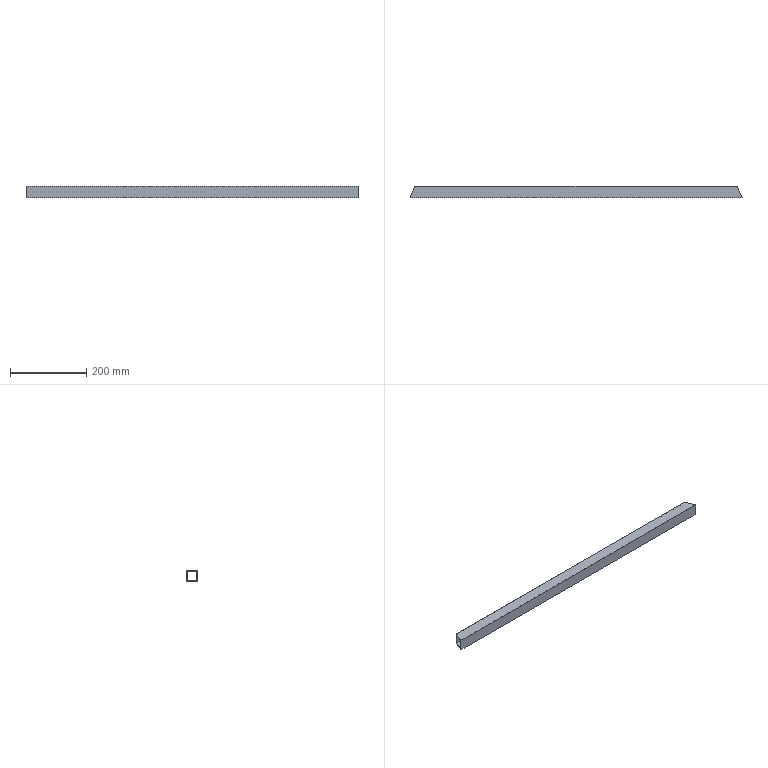Part | NX | features solid 2 | 1 solid | 10 faces | box 870 x 30 x 30 mm | volume 192096 mm3 | plane 10
STEP:
#1=CARTESIAN_POINT('',(422.574,270.,-110.));
#2=VERTEX_POINT('',#1);
#3=CARTESIAN_POINT('',(422.574,270.,-140.));
#4=VERTEX_POINT('',#3);
#5=CARTESIAN_POINT('',(422.574,270.,-110.));
#6=DIRECTION('',(0.,0.,-1.));
#7=VECTOR('',#6,1000.);
#8=LINE('',#5,#7);
#9=EDGE_CURVE('',#2,#4,#8,.T.);
#10=ORIENTED_EDGE('',*,*,#9,.T.);
#11=CARTESIAN_POINT('',(-422.574,270.,-140.));
#12=VERTEX_POINT('',#11);
#13=CARTESIAN_POINT('',(435.,270.,-140.));
#14=DIRECTION('',(-1.,0.,0.));
#15=VECTOR('',#14,1000.);
#16=LINE('',#13,#15);
#17=EDGE_CURVE('',#4,#12,#16,.T.);
#18=ORIENTED_EDGE('',*,*,#17,.T.);
#19=CARTESIAN_POINT('',(-422.574,270.,-110.));
#20=VERTEX_POINT('',#19);
#21=CARTESIAN_POINT('',(-422.574,270.,-110.));
#22=DIRECTION('',(0.,0.,-1.));
#23=VECTOR('',#22,1000.);
#24=LINE('',#21,#23);
#25=EDGE_CURVE('',#20,#12,#24,.T.);
#26=ORIENTED_EDGE('',*,*,#25,.F.);
#27=CARTESIAN_POINT('',(435.,270.,-110.));
#28=DIRECTION('',(-1.,0.,0.));
#29=VECTOR('',#28,1000.);
#30=LINE('',#27,#29);
#31=EDGE_CURVE('',#2,#20,#30,.T.);
#32=ORIENTED_EDGE('',*,*,#31,.F.);
#33=EDGE_LOOP('',(#10,#18,#26,#32));
#34=FACE_BOUND('',#33,.T.);
#35=CARTESIAN_POINT('',(435.,270.,-110.));
#36=DIRECTION('',(0.,1.,0.));
#37=DIRECTION('',(0.,0.,1.));
#38=AXIS2_PLACEMENT_3D('',#35,#36,#37);
#39=PLANE('',#38);
#40=ADVANCED_FACE('',(#34),#39,.T.);
#41=CARTESIAN_POINT('',(435.,240.,-140.));
#42=VERTEX_POINT('',#41);
#43=CARTESIAN_POINT('',(-435.,240.,-140.));
#44=VERTEX_POINT('',#43);
#45=CARTESIAN_POINT('',(435.,240.,-140.));
#46=DIRECTION('',(-1.,0.,0.));
#47=VECTOR('',#46,1000.);
#48=LINE('',#45,#47);
#49=EDGE_CURVE('',#42,#44,#48,.T.);
#50=ORIENTED_EDGE('',*,*,#49,.F.);
#51=CARTESIAN_POINT('',(435.,240.,-110.));
#52=VERTEX_POINT('',#51);
#53=CARTESIAN_POINT('',(435.,240.,-110.));
#54=DIRECTION('',(0.,0.,-1.));
#55=VECTOR('',#54,1000.);
#56=LINE('',#53,#55);
#57=EDGE_CURVE('',#52,#42,#56,.T.);
#58=ORIENTED_EDGE('',*,*,#57,.F.);
#59=CARTESIAN_POINT('',(-435.,240.,-110.));
#60=VERTEX_POINT('',#59);
#61=CARTESIAN_POINT('',(435.,240.,-110.));
#62=DIRECTION('',(-1.,0.,0.));
#63=VECTOR('',#62,1000.);
#64=LINE('',#61,#63);
#65=EDGE_CURVE('',#52,#60,#64,.T.);
#66=ORIENTED_EDGE('',*,*,#65,.T.);
#67=CARTESIAN_POINT('',(-435.,240.,-110.));
#68=DIRECTION('',(0.,0.,-1.));
#69=VECTOR('',#68,1000.);
#70=LINE('',#67,#69);
#71=EDGE_CURVE('',#60,#44,#70,.T.);
#72=ORIENTED_EDGE('',*,*,#71,.T.);
#73=EDGE_LOOP('',(#50,#58,#66,#72));
#74=FACE_BOUND('',#73,.T.);
#75=CARTESIAN_POINT('',(435.,240.,-110.));
#76=DIRECTION('',(0.,1.,0.));
#77=DIRECTION('',(0.,0.,1.));
#78=AXIS2_PLACEMENT_3D('',#75,#76,#77);
#79=PLANE('',#78);
#80=ADVANCED_FACE('',(#74),#79,.F.);
#81=ORIENTED_EDGE('',*,*,#31,.T.);
#82=CARTESIAN_POINT('',(-424.393,265.607,-110.));
#83=DIRECTION('',(-0.3827,-0.9239,0.));
#84=VECTOR('',#83,1000.);
#85=LINE('',#82,#84);
#86=EDGE_CURVE('',#20,#60,#85,.T.);
#87=ORIENTED_EDGE('',*,*,#86,.T.);
#88=ORIENTED_EDGE('',*,*,#65,.F.);
#89=CARTESIAN_POINT('',(424.393,265.607,-110.));
#90=DIRECTION('',(0.3827,-0.9239,0.));
#91=VECTOR('',#90,1000.);
#92=LINE('',#89,#91);
#93=EDGE_CURVE('',#2,#52,#92,.T.);
#94=ORIENTED_EDGE('',*,*,#93,.F.);
#95=EDGE_LOOP('',(#81,#87,#88,#94));
#96=FACE_BOUND('',#95,.T.);
#97=CARTESIAN_POINT('',(435.,270.,-110.));
#98=DIRECTION('',(0.,0.,-1.));
#99=DIRECTION('',(1.,0.,0.));
#100=AXIS2_PLACEMENT_3D('',#97,#98,#99);
#101=PLANE('',#100);
#102=ADVANCED_FACE('',(#96),#101,.F.);
#103=CARTESIAN_POINT('',(424.393,265.607,-140.));
#104=DIRECTION('',(0.3827,-0.9239,0.));
#105=VECTOR('',#104,1000.);
#106=LINE('',#103,#105);
#107=EDGE_CURVE('',#4,#42,#106,.T.);
#108=ORIENTED_EDGE('',*,*,#107,.T.);
#109=ORIENTED_EDGE('',*,*,#49,.T.);
#110=CARTESIAN_POINT('',(-424.393,265.607,-140.));
#111=DIRECTION('',(-0.3827,-0.9239,0.));
#112=VECTOR('',#111,1000.);
#113=LINE('',#110,#112);
#114=EDGE_CURVE('',#12,#44,#113,.T.);
#115=ORIENTED_EDGE('',*,*,#114,.F.);
#116=ORIENTED_EDGE('',*,*,#17,.F.);
#117=EDGE_LOOP('',(#108,#109,#115,#116));
#118=FACE_BOUND('',#117,.T.);
#119=CARTESIAN_POINT('',(435.,270.,-140.));
#120=DIRECTION('',(0.,0.,-1.));
#121=DIRECTION('',(1.,0.,0.));
#122=AXIS2_PLACEMENT_3D('',#119,#120,#121);
#123=PLANE('',#122);
#124=ADVANCED_FACE('',(#118),#123,.T.);
#125=CARTESIAN_POINT('',(423.402,268.,-112.));
#126=VERTEX_POINT('',#125);
#127=CARTESIAN_POINT('',(-423.402,268.,-112.));
#128=VERTEX_POINT('',#127);
#129=CARTESIAN_POINT('',(435.,268.,-112.));
#130=DIRECTION('',(-1.,0.,0.));
#131=VECTOR('',#130,1000.);
#132=LINE('',#129,#131);
#133=EDGE_CURVE('',#126,#128,#132,.T.);
#134=ORIENTED_EDGE('',*,*,#133,.T.);
#135=CARTESIAN_POINT('',(-423.402,268.,-138.));
#136=VERTEX_POINT('',#135);
#137=CARTESIAN_POINT('',(-423.402,268.,-110.));
#138=DIRECTION('',(0.,0.,-1.));
#139=VECTOR('',#138,1000.);
#140=LINE('',#137,#139);
#141=EDGE_CURVE('',#128,#136,#140,.T.);
#142=ORIENTED_EDGE('',*,*,#141,.T.);
#143=CARTESIAN_POINT('',(423.402,268.,-138.));
#144=VERTEX_POINT('',#143);
#145=CARTESIAN_POINT('',(435.,268.,-138.));
#146=DIRECTION('',(-1.,0.,0.));
#147=VECTOR('',#146,1000.);
#148=LINE('',#145,#147);
#149=EDGE_CURVE('',#144,#136,#148,.T.);
#150=ORIENTED_EDGE('',*,*,#149,.F.);
#151=CARTESIAN_POINT('',(423.402,268.,-110.));
#152=DIRECTION('',(0.,0.,-1.));
#153=VECTOR('',#152,1000.);
#154=LINE('',#151,#153);
#155=EDGE_CURVE('',#126,#144,#154,.T.);
#156=ORIENTED_EDGE('',*,*,#155,.F.);
#157=EDGE_LOOP('',(#134,#142,#150,#156));
#158=FACE_BOUND('',#157,.T.);
#159=CARTESIAN_POINT('',(435.,268.,-110.));
#160=DIRECTION('',(0.,1.,0.));
#161=DIRECTION('',(0.,0.,1.));
#162=AXIS2_PLACEMENT_3D('',#159,#160,#161);
#163=PLANE('',#162);
#164=ADVANCED_FACE('',(#158),#163,.F.);
#165=CARTESIAN_POINT('',(434.172,242.,-112.));
#166=VERTEX_POINT('',#165);
#167=CARTESIAN_POINT('',(434.172,242.,-138.));
#168=VERTEX_POINT('',#167);
#169=CARTESIAN_POINT('',(434.172,242.,-110.));
#170=DIRECTION('',(0.,0.,-1.));
#171=VECTOR('',#170,1000.);
#172=LINE('',#169,#171);
#173=EDGE_CURVE('',#166,#168,#172,.T.);
#174=ORIENTED_EDGE('',*,*,#173,.T.);
#175=CARTESIAN_POINT('',(-434.172,242.,-138.));
#176=VERTEX_POINT('',#175);
#177=CARTESIAN_POINT('',(435.,242.,-138.));
#178=DIRECTION('',(-1.,0.,0.));
#179=VECTOR('',#178,1000.);
#180=LINE('',#177,#179);
#181=EDGE_CURVE('',#168,#176,#180,.T.);
#182=ORIENTED_EDGE('',*,*,#181,.T.);
#183=CARTESIAN_POINT('',(-434.172,242.,-112.));
#184=VERTEX_POINT('',#183);
#185=CARTESIAN_POINT('',(-434.172,242.,-110.));
#186=DIRECTION('',(0.,0.,-1.));
#187=VECTOR('',#186,1000.);
#188=LINE('',#185,#187);
#189=EDGE_CURVE('',#184,#176,#188,.T.);
#190=ORIENTED_EDGE('',*,*,#189,.F.);
#191=CARTESIAN_POINT('',(435.,242.,-112.));
#192=DIRECTION('',(-1.,0.,0.));
#193=VECTOR('',#192,1000.);
#194=LINE('',#191,#193);
#195=EDGE_CURVE('',#166,#184,#194,.T.);
#196=ORIENTED_EDGE('',*,*,#195,.F.);
#197=EDGE_LOOP('',(#174,#182,#190,#196));
#198=FACE_BOUND('',#197,.T.);
#199=CARTESIAN_POINT('',(435.,242.,-110.));
#200=DIRECTION('',(0.,1.,0.));
#201=DIRECTION('',(0.,0.,1.));
#202=AXIS2_PLACEMENT_3D('',#199,#200,#201);
#203=PLANE('',#202);
#204=ADVANCED_FACE('',(#198),#203,.T.);
#205=CARTESIAN_POINT('',(424.393,265.607,-112.));
#206=DIRECTION('',(0.3827,-0.9239,0.));
#207=VECTOR('',#206,1000.);
#208=LINE('',#205,#207);
#209=EDGE_CURVE('',#126,#166,#208,.T.);
#210=ORIENTED_EDGE('',*,*,#209,.T.);
#211=ORIENTED_EDGE('',*,*,#195,.T.);
#212=CARTESIAN_POINT('',(-424.393,265.607,-112.));
#213=DIRECTION('',(-0.3827,-0.9239,0.));
#214=VECTOR('',#213,1000.);
#215=LINE('',#212,#214);
#216=EDGE_CURVE('',#128,#184,#215,.T.);
#217=ORIENTED_EDGE('',*,*,#216,.F.);
#218=ORIENTED_EDGE('',*,*,#133,.F.);
#219=EDGE_LOOP('',(#210,#211,#217,#218));
#220=FACE_BOUND('',#219,.T.);
#221=CARTESIAN_POINT('',(435.,270.,-112.));
#222=DIRECTION('',(0.,0.,-1.));
#223=DIRECTION('',(1.,0.,0.));
#224=AXIS2_PLACEMENT_3D('',#221,#222,#223);
#225=PLANE('',#224);
#226=ADVANCED_FACE('',(#220),#225,.T.);
#227=ORIENTED_EDGE('',*,*,#149,.T.);
#228=CARTESIAN_POINT('',(-424.393,265.607,-138.));
#229=DIRECTION('',(-0.3827,-0.9239,0.));
#230=VECTOR('',#229,1000.);
#231=LINE('',#228,#230);
#232=EDGE_CURVE('',#136,#176,#231,.T.);
#233=ORIENTED_EDGE('',*,*,#232,.T.);
#234=ORIENTED_EDGE('',*,*,#181,.F.);
#235=CARTESIAN_POINT('',(424.393,265.607,-138.));
#236=DIRECTION('',(0.3827,-0.9239,0.));
#237=VECTOR('',#236,1000.);
#238=LINE('',#235,#237);
#239=EDGE_CURVE('',#144,#168,#238,.T.);
#240=ORIENTED_EDGE('',*,*,#239,.F.);
#241=EDGE_LOOP('',(#227,#233,#234,#240));
#242=FACE_BOUND('',#241,.T.);
#243=CARTESIAN_POINT('',(435.,270.,-138.));
#244=DIRECTION('',(0.,0.,-1.));
#245=DIRECTION('',(1.,0.,0.));
#246=AXIS2_PLACEMENT_3D('',#243,#244,#245);
#247=PLANE('',#246);
#248=ADVANCED_FACE('',(#242),#247,.F.);
#249=ORIENTED_EDGE('',*,*,#155,.T.);
#250=ORIENTED_EDGE('',*,*,#239,.T.);
#251=ORIENTED_EDGE('',*,*,#173,.F.);
#252=ORIENTED_EDGE('',*,*,#209,.F.);
#253=EDGE_LOOP('',(#249,#250,#251,#252));
#254=FACE_BOUND('',#253,.T.);
#255=ORIENTED_EDGE('',*,*,#93,.T.);
#256=ORIENTED_EDGE('',*,*,#57,.T.);
#257=ORIENTED_EDGE('',*,*,#107,.F.);
#258=ORIENTED_EDGE('',*,*,#9,.F.);
#259=EDGE_LOOP('',(#255,#256,#257,#258));
#260=FACE_BOUND('',#259,.T.);
#261=CARTESIAN_POINT('',(435.,240.,-110.));
#262=DIRECTION('',(-0.9239,-0.3827,0.));
#263=DIRECTION('',(-0.3827,0.9239,0.));
#264=AXIS2_PLACEMENT_3D('',#261,#262,#263);
#265=PLANE('',#264);
#266=ADVANCED_FACE('',(#254,#260),#265,.F.);
#267=ORIENTED_EDGE('',*,*,#141,.F.);
#268=ORIENTED_EDGE('',*,*,#216,.T.);
#269=ORIENTED_EDGE('',*,*,#189,.T.);
#270=ORIENTED_EDGE('',*,*,#232,.F.);
#271=EDGE_LOOP('',(#267,#268,#269,#270));
#272=FACE_BOUND('',#271,.T.);
#273=ORIENTED_EDGE('',*,*,#86,.F.);
#274=ORIENTED_EDGE('',*,*,#25,.T.);
#275=ORIENTED_EDGE('',*,*,#114,.T.);
#276=ORIENTED_EDGE('',*,*,#71,.F.);
#277=EDGE_LOOP('',(#273,#274,#275,#276));
#278=FACE_BOUND('',#277,.T.);
#279=CARTESIAN_POINT('',(-435.,240.,-110.));
#280=DIRECTION('',(0.9239,-0.3827,0.));
#281=DIRECTION('',(0.3827,0.9239,0.));
#282=AXIS2_PLACEMENT_3D('',#279,#280,#281);
#283=PLANE('',#282);
#284=ADVANCED_FACE('',(#272,#278),#283,.F.);
#285=CLOSED_SHELL('',(#40,#80,#102,#124,#164,#204,#226,#248,#266,#284));
#286=MANIFOLD_SOLID_BREP('',#285);
#287=(LENGTH_UNIT()NAMED_UNIT(*)SI_UNIT(.MILLI.,.METRE.));
#288=UNCERTAINTY_MEASURE_WITH_UNIT(LENGTH_MEASURE(0.00001),#287,'','');
#289=(NAMED_UNIT(*)PLANE_ANGLE_UNIT()SI_UNIT($,.RADIAN.));
#290=(NAMED_UNIT(*)SI_UNIT($,.STERADIAN.)SOLID_ANGLE_UNIT());
#291=(GEOMETRIC_REPRESENTATION_CONTEXT(3)GLOBAL_UNCERTAINTY_ASSIGNED_CONTEXT((#288))GLOBAL_UNIT_ASSIGNED_CONTEXT((#287,#289,#290))REPRESENTATION_CONTEXT('',''));
#292=ADVANCED_BREP_SHAPE_REPRESENTATION('',(#286),#291);